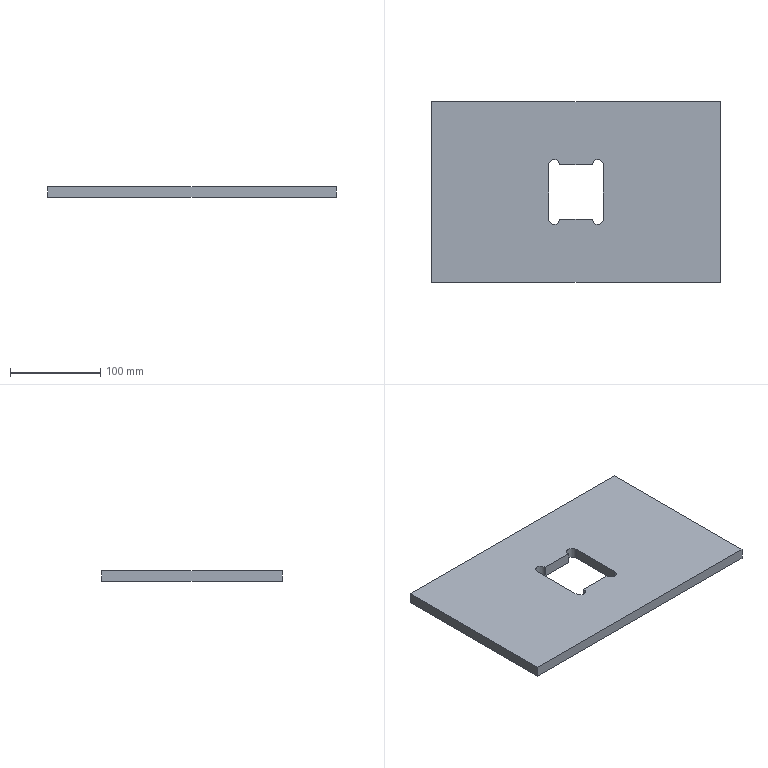Part | SolidWorks | features BaseBody 1 | 1 solid | 14 faces | box 320 x 200 x 12 mm | volume 721363 mm3 | plane 10 | cylinder 4 | commonest cylinder face diameters 12 x4
STEP:
#1=CARTESIAN_POINT('',(30.25,-30.25,0.));
#2=VERTEX_POINT('',#1);
#3=CARTESIAN_POINT('',(30.25,-30.25,12.));
#4=VERTEX_POINT('',#3);
#5=CARTESIAN_POINT('',(30.25,-30.25,-0.001));
#6=DIRECTION('',(0.,0.,1.));
#7=VECTOR('',#6,1000.);
#8=LINE('',#5,#7);
#9=EDGE_CURVE('',#2,#4,#8,.T.);
#10=ORIENTED_EDGE('',*,*,#9,.F.);
#11=CARTESIAN_POINT('',(18.25,-30.25,0.));
#12=VERTEX_POINT('',#11);
#13=CARTESIAN_POINT('',(24.25,-30.25,0.));
#14=DIRECTION('',(0.,0.,1.));
#15=DIRECTION('',(-1.,0.,0.));
#16=AXIS2_PLACEMENT_3D('',#13,#14,#15);
#17=CIRCLE('',#16,6.);
#18=EDGE_CURVE('',#12,#2,#17,.T.);
#19=ORIENTED_EDGE('',*,*,#18,.F.);
#20=CARTESIAN_POINT('',(18.25,-30.25,12.));
#21=VERTEX_POINT('',#20);
#22=CARTESIAN_POINT('',(18.25,-30.25,-0.001));
#23=DIRECTION('',(0.,0.,1.));
#24=VECTOR('',#23,1000.);
#25=LINE('',#22,#24);
#26=EDGE_CURVE('',#12,#21,#25,.T.);
#27=ORIENTED_EDGE('',*,*,#26,.T.);
#28=CARTESIAN_POINT('',(24.25,-30.25,12.));
#29=DIRECTION('',(0.,0.,1.));
#30=DIRECTION('',(1.,0.,0.));
#31=AXIS2_PLACEMENT_3D('',#28,#29,#30);
#32=CIRCLE('',#31,6.);
#33=EDGE_CURVE('',#21,#4,#32,.T.);
#34=ORIENTED_EDGE('',*,*,#33,.T.);
#35=EDGE_LOOP('',(#10,#19,#27,#34));
#36=FACE_OUTER_BOUND('',#35,.T.);
#37=CARTESIAN_POINT('',(24.25,-30.25,-0.001));
#38=DIRECTION('',(0.,0.,1.));
#39=DIRECTION('',(1.,0.,0.));
#40=AXIS2_PLACEMENT_3D('',#37,#38,#39);
#41=CYLINDRICAL_SURFACE('',#40,6.);
#42=ADVANCED_FACE('',(#36),#41,.F.);
#43=CARTESIAN_POINT('',(-18.25,-30.25,12.));
#44=VERTEX_POINT('',#43);
#45=CARTESIAN_POINT('',(-18.25,-30.25,0.));
#46=VERTEX_POINT('',#45);
#47=CARTESIAN_POINT('',(-18.25,-30.25,-0.001));
#48=DIRECTION('',(0.,0.,-1.));
#49=VECTOR('',#48,1000.);
#50=LINE('',#47,#49);
#51=EDGE_CURVE('',#44,#46,#50,.T.);
#52=ORIENTED_EDGE('',*,*,#51,.T.);
#53=CARTESIAN_POINT('',(-30.25,-30.25,0.));
#54=VERTEX_POINT('',#53);
#55=CARTESIAN_POINT('',(-24.25,-30.25,0.));
#56=DIRECTION('',(0.,0.,1.));
#57=DIRECTION('',(-1.,0.,0.));
#58=AXIS2_PLACEMENT_3D('',#55,#56,#57);
#59=CIRCLE('',#58,6.);
#60=EDGE_CURVE('',#54,#46,#59,.T.);
#61=ORIENTED_EDGE('',*,*,#60,.F.);
#62=CARTESIAN_POINT('',(-30.25,-30.25,12.));
#63=VERTEX_POINT('',#62);
#64=CARTESIAN_POINT('',(-30.25,-30.25,-0.001));
#65=DIRECTION('',(0.,0.,1.));
#66=VECTOR('',#65,1000.);
#67=LINE('',#64,#66);
#68=EDGE_CURVE('',#54,#63,#67,.T.);
#69=ORIENTED_EDGE('',*,*,#68,.T.);
#70=CARTESIAN_POINT('',(-24.25,-30.25,12.));
#71=DIRECTION('',(0.,0.,1.));
#72=DIRECTION('',(1.,0.,0.));
#73=AXIS2_PLACEMENT_3D('',#70,#71,#72);
#74=CIRCLE('',#73,6.);
#75=EDGE_CURVE('',#63,#44,#74,.T.);
#76=ORIENTED_EDGE('',*,*,#75,.T.);
#77=EDGE_LOOP('',(#52,#61,#69,#76));
#78=FACE_OUTER_BOUND('',#77,.T.);
#79=CARTESIAN_POINT('',(-24.25,-30.25,-0.001));
#80=DIRECTION('',(0.,0.,1.));
#81=DIRECTION('',(1.,0.,0.));
#82=AXIS2_PLACEMENT_3D('',#79,#80,#81);
#83=CYLINDRICAL_SURFACE('',#82,6.);
#84=ADVANCED_FACE('',(#78),#83,.F.);
#85=CARTESIAN_POINT('',(18.25,30.25,12.));
#86=VERTEX_POINT('',#85);
#87=CARTESIAN_POINT('',(18.25,30.25,0.));
#88=VERTEX_POINT('',#87);
#89=CARTESIAN_POINT('',(18.25,30.25,-0.001));
#90=DIRECTION('',(0.,0.,-1.));
#91=VECTOR('',#90,1000.);
#92=LINE('',#89,#91);
#93=EDGE_CURVE('',#86,#88,#92,.T.);
#94=ORIENTED_EDGE('',*,*,#93,.T.);
#95=CARTESIAN_POINT('',(30.25,30.25,0.));
#96=VERTEX_POINT('',#95);
#97=CARTESIAN_POINT('',(24.25,30.25,0.));
#98=DIRECTION('',(0.,0.,1.));
#99=DIRECTION('',(-1.,0.,0.));
#100=AXIS2_PLACEMENT_3D('',#97,#98,#99);
#101=CIRCLE('',#100,6.);
#102=EDGE_CURVE('',#96,#88,#101,.T.);
#103=ORIENTED_EDGE('',*,*,#102,.F.);
#104=CARTESIAN_POINT('',(30.25,30.25,12.));
#105=VERTEX_POINT('',#104);
#106=CARTESIAN_POINT('',(30.25,30.25,-0.001));
#107=DIRECTION('',(0.,0.,1.));
#108=VECTOR('',#107,1000.);
#109=LINE('',#106,#108);
#110=EDGE_CURVE('',#96,#105,#109,.T.);
#111=ORIENTED_EDGE('',*,*,#110,.T.);
#112=CARTESIAN_POINT('',(24.25,30.25,12.));
#113=DIRECTION('',(0.,0.,1.));
#114=DIRECTION('',(1.,0.,0.));
#115=AXIS2_PLACEMENT_3D('',#112,#113,#114);
#116=CIRCLE('',#115,6.);
#117=EDGE_CURVE('',#105,#86,#116,.T.);
#118=ORIENTED_EDGE('',*,*,#117,.T.);
#119=EDGE_LOOP('',(#94,#103,#111,#118));
#120=FACE_OUTER_BOUND('',#119,.T.);
#121=CARTESIAN_POINT('',(24.25,30.25,-0.001));
#122=DIRECTION('',(0.,0.,1.));
#123=DIRECTION('',(1.,0.,0.));
#124=AXIS2_PLACEMENT_3D('',#121,#122,#123);
#125=CYLINDRICAL_SURFACE('',#124,6.);
#126=ADVANCED_FACE('',(#120),#125,.F.);
#127=CARTESIAN_POINT('',(-30.25,30.25,0.));
#128=VERTEX_POINT('',#127);
#129=CARTESIAN_POINT('',(-30.25,30.25,12.));
#130=VERTEX_POINT('',#129);
#131=CARTESIAN_POINT('',(-30.25,30.25,-0.001));
#132=DIRECTION('',(0.,0.,1.));
#133=VECTOR('',#132,1000.);
#134=LINE('',#131,#133);
#135=EDGE_CURVE('',#128,#130,#134,.T.);
#136=ORIENTED_EDGE('',*,*,#135,.F.);
#137=CARTESIAN_POINT('',(-18.25,30.25,0.));
#138=VERTEX_POINT('',#137);
#139=CARTESIAN_POINT('',(-24.25,30.25,0.));
#140=DIRECTION('',(0.,0.,1.));
#141=DIRECTION('',(-1.,0.,0.));
#142=AXIS2_PLACEMENT_3D('',#139,#140,#141);
#143=CIRCLE('',#142,6.);
#144=EDGE_CURVE('',#138,#128,#143,.T.);
#145=ORIENTED_EDGE('',*,*,#144,.F.);
#146=CARTESIAN_POINT('',(-18.25,30.25,12.));
#147=VERTEX_POINT('',#146);
#148=CARTESIAN_POINT('',(-18.25,30.25,-0.001));
#149=DIRECTION('',(0.,0.,1.));
#150=VECTOR('',#149,1000.);
#151=LINE('',#148,#150);
#152=EDGE_CURVE('',#138,#147,#151,.T.);
#153=ORIENTED_EDGE('',*,*,#152,.T.);
#154=CARTESIAN_POINT('',(-24.25,30.25,12.));
#155=DIRECTION('',(0.,0.,1.));
#156=DIRECTION('',(1.,0.,0.));
#157=AXIS2_PLACEMENT_3D('',#154,#155,#156);
#158=CIRCLE('',#157,6.);
#159=EDGE_CURVE('',#147,#130,#158,.T.);
#160=ORIENTED_EDGE('',*,*,#159,.T.);
#161=EDGE_LOOP('',(#136,#145,#153,#160));
#162=FACE_OUTER_BOUND('',#161,.T.);
#163=CARTESIAN_POINT('',(-24.25,30.25,-0.001));
#164=DIRECTION('',(0.,0.,1.));
#165=DIRECTION('',(1.,0.,0.));
#166=AXIS2_PLACEMENT_3D('',#163,#164,#165);
#167=CYLINDRICAL_SURFACE('',#166,6.);
#168=ADVANCED_FACE('',(#162),#167,.F.);
#169=CARTESIAN_POINT('',(-30.25,30.25,0.));
#170=DIRECTION('',(-1.,0.,0.));
#171=VECTOR('',#170,1000.);
#172=LINE('',#169,#171);
#173=EDGE_CURVE('',#88,#138,#172,.T.);
#174=ORIENTED_EDGE('',*,*,#173,.F.);
#175=ORIENTED_EDGE('',*,*,#93,.F.);
#176=CARTESIAN_POINT('',(-30.25,30.25,12.));
#177=DIRECTION('',(-1.,0.,0.));
#178=VECTOR('',#177,1000.);
#179=LINE('',#176,#178);
#180=EDGE_CURVE('',#86,#147,#179,.T.);
#181=ORIENTED_EDGE('',*,*,#180,.T.);
#182=ORIENTED_EDGE('',*,*,#152,.F.);
#183=EDGE_LOOP('',(#174,#175,#181,#182));
#184=FACE_OUTER_BOUND('',#183,.T.);
#185=CARTESIAN_POINT('',(-30.25,30.25,-0.001));
#186=DIRECTION('',(0.,1.,0.));
#187=DIRECTION('',(1.,0.,0.));
#188=AXIS2_PLACEMENT_3D('',#185,#186,#187);
#189=PLANE('',#188);
#190=ADVANCED_FACE('',(#184),#189,.F.);
#191=ORIENTED_EDGE('',*,*,#135,.T.);
#192=CARTESIAN_POINT('',(-30.25,-30.25,12.));
#193=DIRECTION('',(0.,-1.,0.));
#194=VECTOR('',#193,1000.);
#195=LINE('',#192,#194);
#196=EDGE_CURVE('',#130,#63,#195,.T.);
#197=ORIENTED_EDGE('',*,*,#196,.T.);
#198=ORIENTED_EDGE('',*,*,#68,.F.);
#199=CARTESIAN_POINT('',(-30.25,-30.25,0.));
#200=DIRECTION('',(0.,-1.,0.));
#201=VECTOR('',#200,1000.);
#202=LINE('',#199,#201);
#203=EDGE_CURVE('',#128,#54,#202,.T.);
#204=ORIENTED_EDGE('',*,*,#203,.F.);
#205=EDGE_LOOP('',(#191,#197,#198,#204));
#206=FACE_OUTER_BOUND('',#205,.T.);
#207=CARTESIAN_POINT('',(-30.25,-30.25,-0.001));
#208=DIRECTION('',(-1.,0.,0.));
#209=DIRECTION('',(0.,0.,1.));
#210=AXIS2_PLACEMENT_3D('',#207,#208,#209);
#211=PLANE('',#210);
#212=ADVANCED_FACE('',(#206),#211,.F.);
#213=CARTESIAN_POINT('',(-30.25,-30.25,0.));
#214=DIRECTION('',(1.,0.,0.));
#215=VECTOR('',#214,1000.);
#216=LINE('',#213,#215);
#217=EDGE_CURVE('',#46,#12,#216,.T.);
#218=ORIENTED_EDGE('',*,*,#217,.F.);
#219=ORIENTED_EDGE('',*,*,#51,.F.);
#220=CARTESIAN_POINT('',(-30.25,-30.25,12.));
#221=DIRECTION('',(1.,0.,0.));
#222=VECTOR('',#221,1000.);
#223=LINE('',#220,#222);
#224=EDGE_CURVE('',#44,#21,#223,.T.);
#225=ORIENTED_EDGE('',*,*,#224,.T.);
#226=ORIENTED_EDGE('',*,*,#26,.F.);
#227=EDGE_LOOP('',(#218,#219,#225,#226));
#228=FACE_OUTER_BOUND('',#227,.T.);
#229=CARTESIAN_POINT('',(-30.25,-30.25,-0.001));
#230=DIRECTION('',(0.,-1.,0.));
#231=DIRECTION('',(0.,0.,-1.));
#232=AXIS2_PLACEMENT_3D('',#229,#230,#231);
#233=PLANE('',#232);
#234=ADVANCED_FACE('',(#228),#233,.F.);
#235=ORIENTED_EDGE('',*,*,#9,.T.);
#236=CARTESIAN_POINT('',(30.25,-30.25,12.));
#237=DIRECTION('',(0.,1.,0.));
#238=VECTOR('',#237,1000.);
#239=LINE('',#236,#238);
#240=EDGE_CURVE('',#4,#105,#239,.T.);
#241=ORIENTED_EDGE('',*,*,#240,.T.);
#242=ORIENTED_EDGE('',*,*,#110,.F.);
#243=CARTESIAN_POINT('',(30.25,-30.25,0.));
#244=DIRECTION('',(0.,1.,0.));
#245=VECTOR('',#244,1000.);
#246=LINE('',#243,#245);
#247=EDGE_CURVE('',#2,#96,#246,.T.);
#248=ORIENTED_EDGE('',*,*,#247,.F.);
#249=EDGE_LOOP('',(#235,#241,#242,#248));
#250=FACE_OUTER_BOUND('',#249,.T.);
#251=CARTESIAN_POINT('',(30.25,-30.25,-0.001));
#252=DIRECTION('',(1.,0.,0.));
#253=DIRECTION('',(0.,1.,0.));
#254=AXIS2_PLACEMENT_3D('',#251,#252,#253);
#255=PLANE('',#254);
#256=ADVANCED_FACE('',(#250),#255,.F.);
#257=ORIENTED_EDGE('',*,*,#102,.T.);
#258=ORIENTED_EDGE('',*,*,#173,.T.);
#259=ORIENTED_EDGE('',*,*,#144,.T.);
#260=ORIENTED_EDGE('',*,*,#203,.T.);
#261=ORIENTED_EDGE('',*,*,#60,.T.);
#262=ORIENTED_EDGE('',*,*,#217,.T.);
#263=ORIENTED_EDGE('',*,*,#18,.T.);
#264=ORIENTED_EDGE('',*,*,#247,.T.);
#265=EDGE_LOOP('',(#257,#258,#259,#260,#261,#262,#263,#264));
#266=FACE_BOUND('',#265,.T.);
#267=CARTESIAN_POINT('',(160.,-100.,0.));
#268=VERTEX_POINT('',#267);
#269=CARTESIAN_POINT('',(160.,100.,0.));
#270=VERTEX_POINT('',#269);
#271=CARTESIAN_POINT('',(160.,-100.,0.));
#272=DIRECTION('',(0.,1.,0.));
#273=VECTOR('',#272,1000.);
#274=LINE('',#271,#273);
#275=EDGE_CURVE('',#268,#270,#274,.T.);
#276=ORIENTED_EDGE('',*,*,#275,.F.);
#277=CARTESIAN_POINT('',(-160.,-100.,0.));
#278=VERTEX_POINT('',#277);
#279=CARTESIAN_POINT('',(-160.,-100.,0.));
#280=DIRECTION('',(1.,0.,0.));
#281=VECTOR('',#280,1000.);
#282=LINE('',#279,#281);
#283=EDGE_CURVE('',#278,#268,#282,.T.);
#284=ORIENTED_EDGE('',*,*,#283,.F.);
#285=CARTESIAN_POINT('',(-160.,100.,0.));
#286=VERTEX_POINT('',#285);
#287=CARTESIAN_POINT('',(-160.,-100.,0.));
#288=DIRECTION('',(0.,-1.,0.));
#289=VECTOR('',#288,1000.);
#290=LINE('',#287,#289);
#291=EDGE_CURVE('',#286,#278,#290,.T.);
#292=ORIENTED_EDGE('',*,*,#291,.F.);
#293=CARTESIAN_POINT('',(-160.,100.,0.));
#294=DIRECTION('',(-1.,0.,0.));
#295=VECTOR('',#294,1000.);
#296=LINE('',#293,#295);
#297=EDGE_CURVE('',#270,#286,#296,.T.);
#298=ORIENTED_EDGE('',*,*,#297,.F.);
#299=EDGE_LOOP('',(#276,#284,#292,#298));
#300=FACE_OUTER_BOUND('',#299,.T.);
#301=CARTESIAN_POINT('',(0.,0.,0.));
#302=DIRECTION('',(0.,0.,-1.));
#303=DIRECTION('',(0.,-1.,0.));
#304=AXIS2_PLACEMENT_3D('',#301,#302,#303);
#305=PLANE('',#304);
#306=ADVANCED_FACE('',(#266,#300),#305,.T.);
#307=ORIENTED_EDGE('',*,*,#180,.F.);
#308=ORIENTED_EDGE('',*,*,#117,.F.);
#309=ORIENTED_EDGE('',*,*,#240,.F.);
#310=ORIENTED_EDGE('',*,*,#33,.F.);
#311=ORIENTED_EDGE('',*,*,#224,.F.);
#312=ORIENTED_EDGE('',*,*,#75,.F.);
#313=ORIENTED_EDGE('',*,*,#196,.F.);
#314=ORIENTED_EDGE('',*,*,#159,.F.);
#315=EDGE_LOOP('',(#307,#308,#309,#310,#311,#312,#313,#314));
#316=FACE_BOUND('',#315,.T.);
#317=CARTESIAN_POINT('',(160.,-100.,12.));
#318=VERTEX_POINT('',#317);
#319=CARTESIAN_POINT('',(160.,100.,12.));
#320=VERTEX_POINT('',#319);
#321=CARTESIAN_POINT('',(160.,-100.,12.));
#322=DIRECTION('',(0.,1.,0.));
#323=VECTOR('',#322,1000.);
#324=LINE('',#321,#323);
#325=EDGE_CURVE('',#318,#320,#324,.T.);
#326=ORIENTED_EDGE('',*,*,#325,.T.);
#327=CARTESIAN_POINT('',(-160.,100.,12.));
#328=VERTEX_POINT('',#327);
#329=CARTESIAN_POINT('',(-160.,100.,12.));
#330=DIRECTION('',(-1.,0.,0.));
#331=VECTOR('',#330,1000.);
#332=LINE('',#329,#331);
#333=EDGE_CURVE('',#320,#328,#332,.T.);
#334=ORIENTED_EDGE('',*,*,#333,.T.);
#335=CARTESIAN_POINT('',(-160.,-100.,12.));
#336=VERTEX_POINT('',#335);
#337=CARTESIAN_POINT('',(-160.,-100.,12.));
#338=DIRECTION('',(0.,-1.,0.));
#339=VECTOR('',#338,1000.);
#340=LINE('',#337,#339);
#341=EDGE_CURVE('',#328,#336,#340,.T.);
#342=ORIENTED_EDGE('',*,*,#341,.T.);
#343=CARTESIAN_POINT('',(-160.,-100.,12.));
#344=DIRECTION('',(1.,0.,0.));
#345=VECTOR('',#344,1000.);
#346=LINE('',#343,#345);
#347=EDGE_CURVE('',#336,#318,#346,.T.);
#348=ORIENTED_EDGE('',*,*,#347,.T.);
#349=EDGE_LOOP('',(#326,#334,#342,#348));
#350=FACE_OUTER_BOUND('',#349,.T.);
#351=CARTESIAN_POINT('',(0.,0.,12.));
#352=DIRECTION('',(0.,0.,-1.));
#353=DIRECTION('',(0.,-1.,0.));
#354=AXIS2_PLACEMENT_3D('',#351,#352,#353);
#355=PLANE('',#354);
#356=ADVANCED_FACE('',(#316,#350),#355,.F.);
#357=ORIENTED_EDGE('',*,*,#283,.T.);
#358=CARTESIAN_POINT('',(160.,-100.,12.));
#359=DIRECTION('',(0.,0.,-1.));
#360=VECTOR('',#359,1000.);
#361=LINE('',#358,#360);
#362=EDGE_CURVE('',#318,#268,#361,.T.);
#363=ORIENTED_EDGE('',*,*,#362,.F.);
#364=ORIENTED_EDGE('',*,*,#347,.F.);
#365=CARTESIAN_POINT('',(-160.,-100.,12.));
#366=DIRECTION('',(0.,0.,-1.));
#367=VECTOR('',#366,1000.);
#368=LINE('',#365,#367);
#369=EDGE_CURVE('',#336,#278,#368,.T.);
#370=ORIENTED_EDGE('',*,*,#369,.T.);
#371=EDGE_LOOP('',(#357,#363,#364,#370));
#372=FACE_OUTER_BOUND('',#371,.T.);
#373=CARTESIAN_POINT('',(-160.,-100.,12.));
#374=DIRECTION('',(0.,1.,0.));
#375=DIRECTION('',(1.,0.,0.));
#376=AXIS2_PLACEMENT_3D('',#373,#374,#375);
#377=PLANE('',#376);
#378=ADVANCED_FACE('',(#372),#377,.F.);
#379=ORIENTED_EDGE('',*,*,#291,.T.);
#380=ORIENTED_EDGE('',*,*,#369,.F.);
#381=ORIENTED_EDGE('',*,*,#341,.F.);
#382=CARTESIAN_POINT('',(-160.,100.,12.));
#383=DIRECTION('',(0.,0.,-1.));
#384=VECTOR('',#383,1000.);
#385=LINE('',#382,#384);
#386=EDGE_CURVE('',#328,#286,#385,.T.);
#387=ORIENTED_EDGE('',*,*,#386,.T.);
#388=EDGE_LOOP('',(#379,#380,#381,#387));
#389=FACE_OUTER_BOUND('',#388,.T.);
#390=CARTESIAN_POINT('',(-160.,-100.,12.));
#391=DIRECTION('',(1.,0.,0.));
#392=DIRECTION('',(0.,1.,0.));
#393=AXIS2_PLACEMENT_3D('',#390,#391,#392);
#394=PLANE('',#393);
#395=ADVANCED_FACE('',(#389),#394,.F.);
#396=ORIENTED_EDGE('',*,*,#297,.T.);
#397=ORIENTED_EDGE('',*,*,#386,.F.);
#398=ORIENTED_EDGE('',*,*,#333,.F.);
#399=CARTESIAN_POINT('',(160.,100.,12.));
#400=DIRECTION('',(0.,0.,-1.));
#401=VECTOR('',#400,1000.);
#402=LINE('',#399,#401);
#403=EDGE_CURVE('',#320,#270,#402,.T.);
#404=ORIENTED_EDGE('',*,*,#403,.T.);
#405=EDGE_LOOP('',(#396,#397,#398,#404));
#406=FACE_OUTER_BOUND('',#405,.T.);
#407=CARTESIAN_POINT('',(-160.,100.,12.));
#408=DIRECTION('',(0.,-1.,0.));
#409=DIRECTION('',(0.,0.,-1.));
#410=AXIS2_PLACEMENT_3D('',#407,#408,#409);
#411=PLANE('',#410);
#412=ADVANCED_FACE('',(#406),#411,.F.);
#413=ORIENTED_EDGE('',*,*,#275,.T.);
#414=ORIENTED_EDGE('',*,*,#403,.F.);
#415=ORIENTED_EDGE('',*,*,#325,.F.);
#416=ORIENTED_EDGE('',*,*,#362,.T.);
#417=EDGE_LOOP('',(#413,#414,#415,#416));
#418=FACE_OUTER_BOUND('',#417,.T.);
#419=CARTESIAN_POINT('',(160.,-100.,12.));
#420=DIRECTION('',(-1.,0.,0.));
#421=DIRECTION('',(0.,0.,1.));
#422=AXIS2_PLACEMENT_3D('',#419,#420,#421);
#423=PLANE('',#422);
#424=ADVANCED_FACE('',(#418),#423,.F.);
#425=CLOSED_SHELL('',(#42,#84,#126,#168,#190,#212,#234,#256,#306,#356,#378,#395,#412,#424));
#426=MANIFOLD_SOLID_BREP('',#425);
#427=CARTESIAN_POINT('',(0.,0.,0.));
#428=DIRECTION('',(0.,0.,1.));
#429=DIRECTION('',(1.,0.,0.));
#430=AXIS2_PLACEMENT_3D('',#427,#428,#429);
#431=(LENGTH_UNIT()NAMED_UNIT(*)SI_UNIT(.MILLI.,.METRE.));
#432=UNCERTAINTY_MEASURE_WITH_UNIT(LENGTH_MEASURE(0.00001),#431,'','');
#433=(NAMED_UNIT(*)PLANE_ANGLE_UNIT()SI_UNIT($,.RADIAN.));
#434=(NAMED_UNIT(*)SI_UNIT($,.STERADIAN.)SOLID_ANGLE_UNIT());
#435=(GEOMETRIC_REPRESENTATION_CONTEXT(3)GLOBAL_UNCERTAINTY_ASSIGNED_CONTEXT((#432))GLOBAL_UNIT_ASSIGNED_CONTEXT((#431,#433,#434))REPRESENTATION_CONTEXT('',''));
#436=ADVANCED_BREP_SHAPE_REPRESENTATION('',(#426,#430),#435);